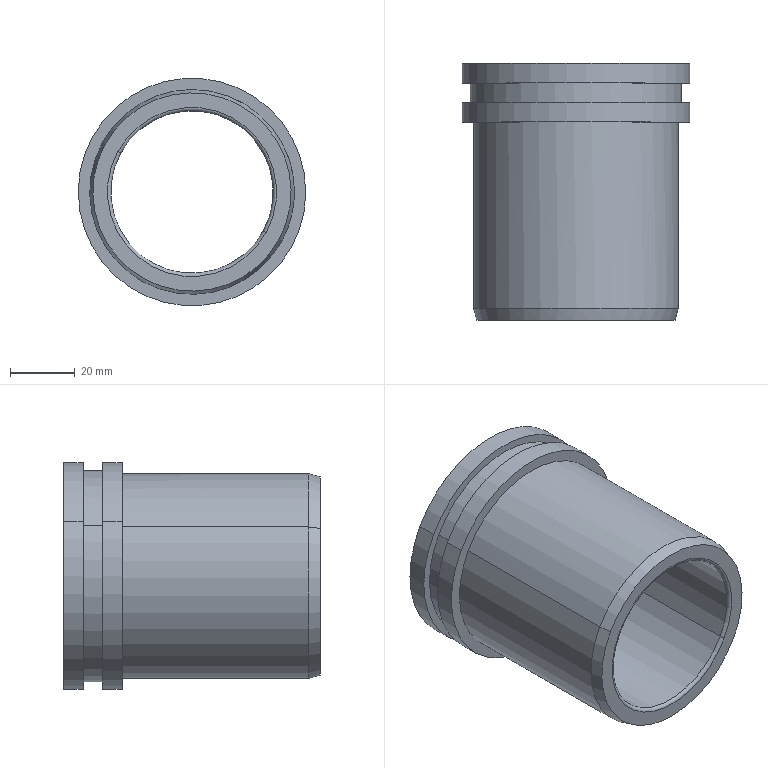Part | CATIA | 1 solid | 21 faces | box 70 x 79 x 70 mm | volume 99847 mm3 | cylinder 10 | plane 5 | torus 4 | cone 2 | commonest cylinder face diameters 70 x4 50 x2 63 x2 65 x2
STEP:
#1=CARTESIAN_POINT('',(-30.715,0.,16.78));
#2=VERTEX_POINT('',#1);
#3=CARTESIAN_POINT('',(-30.715,6.,16.78));
#4=VERTEX_POINT('',#3);
#5=CARTESIAN_POINT('',(-30.715,-21.5,16.78));
#6=DIRECTION('',(0.,1.,0.));
#7=VECTOR('',#6,1.);
#8=LINE('',#5,#7);
#9=EDGE_CURVE('',#2,#4,#8,.T.);
#10=ORIENTED_EDGE('',*,*,#9,.T.);
#11=CARTESIAN_POINT('',(30.715,6.,-16.78));
#12=VERTEX_POINT('',#11);
#13=CARTESIAN_POINT('',(0.,6.,0.));
#14=DIRECTION('',(0.,1.,0.));
#15=AXIS2_PLACEMENT_3D('',#13,#14,$);
#16=CIRCLE('',#15,35.);
#17=EDGE_CURVE('',#12,#4,#16,.T.);
#18=ORIENTED_EDGE('',*,*,#17,.F.);
#19=CARTESIAN_POINT('',(30.715,0.,-16.78));
#20=VERTEX_POINT('',#19);
#21=CARTESIAN_POINT('',(30.715,-21.5,-16.78));
#22=DIRECTION('',(0.,1.,0.));
#23=VECTOR('',#22,1.);
#24=LINE('',#21,#23);
#25=EDGE_CURVE('',#20,#12,#24,.T.);
#26=ORIENTED_EDGE('',*,*,#25,.F.);
#27=CARTESIAN_POINT('',(0.,0.,0.));
#28=DIRECTION('',(0.,1.,0.));
#29=AXIS2_PLACEMENT_3D('',#27,#28,$);
#30=CIRCLE('',#29,35.);
#31=EDGE_CURVE('',#20,#2,#30,.T.);
#32=ORIENTED_EDGE('',*,*,#31,.T.);
#33=EDGE_LOOP('',(#10,#18,#26,#32));
#34=FACE_OUTER_BOUND('',#33,.T.);
#35=CARTESIAN_POINT('',(0.,-21.5,0.));
#36=DIRECTION('',(0.,1.,0.));
#37=DIRECTION('',(0.8776,0.,-0.4794));
#38=AXIS2_PLACEMENT_3D('',#35,#36,#37);
#39=CYLINDRICAL_SURFACE('',#38,35.);
#40=ADVANCED_FACE('',(#34),#39,.T.);
#41=ORIENTED_EDGE('',*,*,#25,.T.);
#42=CARTESIAN_POINT('',(0.,6.,0.));
#43=DIRECTION('',(0.,1.,0.));
#44=AXIS2_PLACEMENT_3D('',#42,#43,$);
#45=CIRCLE('',#44,35.);
#46=EDGE_CURVE('',#4,#12,#45,.T.);
#47=ORIENTED_EDGE('',*,*,#46,.F.);
#48=ORIENTED_EDGE('',*,*,#9,.F.);
#49=CARTESIAN_POINT('',(0.,0.,0.));
#50=DIRECTION('',(0.,1.,0.));
#51=AXIS2_PLACEMENT_3D('',#49,#50,$);
#52=CIRCLE('',#51,35.);
#53=EDGE_CURVE('',#2,#20,#52,.T.);
#54=ORIENTED_EDGE('',*,*,#53,.T.);
#55=EDGE_LOOP('',(#41,#47,#48,#54));
#56=FACE_OUTER_BOUND('',#55,.T.);
#57=CARTESIAN_POINT('',(0.,-21.5,0.));
#58=DIRECTION('',(0.,1.,0.));
#59=DIRECTION('',(-0.8776,0.,0.4794));
#60=AXIS2_PLACEMENT_3D('',#57,#58,#59);
#61=CYLINDRICAL_SURFACE('',#60,35.);
#62=ADVANCED_FACE('',(#56),#61,.T.);
#63=ORIENTED_EDGE('',*,*,#46,.T.);
#64=ORIENTED_EDGE('',*,*,#17,.T.);
#65=EDGE_LOOP('',(#63,#64));
#66=FACE_OUTER_BOUND('',#65,.T.);
#67=CARTESIAN_POINT('',(28.521,6.,-15.581));
#68=VERTEX_POINT('',#67);
#69=CARTESIAN_POINT('',(-28.521,6.,15.581));
#70=VERTEX_POINT('',#69);
#71=CARTESIAN_POINT('',(0.,6.,0.));
#72=DIRECTION('',(0.,1.,0.));
#73=AXIS2_PLACEMENT_3D('',#71,#72,$);
#74=CIRCLE('',#73,32.5);
#75=EDGE_CURVE('',#68,#70,#74,.T.);
#76=ORIENTED_EDGE('',*,*,#75,.F.);
#77=CARTESIAN_POINT('',(0.,6.,0.));
#78=DIRECTION('',(0.,1.,0.));
#79=AXIS2_PLACEMENT_3D('',#77,#78,$);
#80=CIRCLE('',#79,32.5);
#81=EDGE_CURVE('',#70,#68,#80,.T.);
#82=ORIENTED_EDGE('',*,*,#81,.F.);
#83=EDGE_LOOP('',(#76,#82));
#84=FACE_BOUND('',#83,.T.);
#85=CARTESIAN_POINT('',(35.,6.,0.));
#86=DIRECTION('',(0.,1.,0.));
#87=DIRECTION('',(1.,0.,0.));
#88=AXIS2_PLACEMENT_3D('',#85,#86,#87);
#89=PLANE('',#88);
#90=ADVANCED_FACE('',(#66,#84),#89,.T.);
#91=ORIENTED_EDGE('',*,*,#31,.F.);
#92=ORIENTED_EDGE('',*,*,#53,.F.);
#93=EDGE_LOOP('',(#91,#92));
#94=FACE_OUTER_BOUND('',#93,.T.);
#95=CARTESIAN_POINT('',(-27.644,0.,15.102));
#96=VERTEX_POINT('',#95);
#97=CARTESIAN_POINT('',(27.644,0.,-15.102));
#98=VERTEX_POINT('',#97);
#99=CARTESIAN_POINT('',(0.,0.,0.));
#100=DIRECTION('',(0.,1.,0.));
#101=AXIS2_PLACEMENT_3D('',#99,#100,$);
#102=CIRCLE('',#101,31.5);
#103=EDGE_CURVE('',#96,#98,#102,.T.);
#104=ORIENTED_EDGE('',*,*,#103,.T.);
#105=CARTESIAN_POINT('',(0.,0.,0.));
#106=DIRECTION('',(0.,1.,0.));
#107=AXIS2_PLACEMENT_3D('',#105,#106,$);
#108=CIRCLE('',#107,31.5);
#109=EDGE_CURVE('',#98,#96,#108,.T.);
#110=ORIENTED_EDGE('',*,*,#109,.T.);
#111=EDGE_LOOP('',(#104,#110));
#112=FACE_BOUND('',#111,.T.);
#113=CARTESIAN_POINT('',(35.,0.,0.));
#114=DIRECTION('',(0.,1.,0.));
#115=DIRECTION('',(1.,0.,0.));
#116=AXIS2_PLACEMENT_3D('',#113,#114,#115);
#117=PLANE('',#116);
#118=ADVANCED_FACE('',(#94,#112),#117,.F.);
#119=CARTESIAN_POINT('',(-28.521,12.,15.581));
#120=VERTEX_POINT('',#119);
#121=CARTESIAN_POINT('',(-28.521,-21.5,15.581));
#122=DIRECTION('',(0.,1.,0.));
#123=VECTOR('',#122,1.);
#124=LINE('',#121,#123);
#125=EDGE_CURVE('',#70,#120,#124,.T.);
#126=ORIENTED_EDGE('',*,*,#125,.T.);
#127=CARTESIAN_POINT('',(28.521,12.,-15.581));
#128=VERTEX_POINT('',#127);
#129=CARTESIAN_POINT('',(0.,12.,0.));
#130=DIRECTION('',(0.,1.,0.));
#131=AXIS2_PLACEMENT_3D('',#129,#130,$);
#132=CIRCLE('',#131,32.5);
#133=EDGE_CURVE('',#128,#120,#132,.T.);
#134=ORIENTED_EDGE('',*,*,#133,.F.);
#135=CARTESIAN_POINT('',(28.521,-21.5,-15.581));
#136=DIRECTION('',(0.,1.,0.));
#137=VECTOR('',#136,1.);
#138=LINE('',#135,#137);
#139=EDGE_CURVE('',#68,#128,#138,.T.);
#140=ORIENTED_EDGE('',*,*,#139,.F.);
#141=ORIENTED_EDGE('',*,*,#75,.T.);
#142=EDGE_LOOP('',(#126,#134,#140,#141));
#143=FACE_OUTER_BOUND('',#142,.T.);
#144=CARTESIAN_POINT('',(0.,-21.5,0.));
#145=DIRECTION('',(0.,1.,0.));
#146=DIRECTION('',(0.8776,0.,-0.4794));
#147=AXIS2_PLACEMENT_3D('',#144,#145,#146);
#148=CYLINDRICAL_SURFACE('',#147,32.5);
#149=ADVANCED_FACE('',(#143),#148,.T.);
#150=ORIENTED_EDGE('',*,*,#139,.T.);
#151=CARTESIAN_POINT('',(0.,12.,0.));
#152=DIRECTION('',(0.,1.,0.));
#153=AXIS2_PLACEMENT_3D('',#151,#152,$);
#154=CIRCLE('',#153,32.5);
#155=EDGE_CURVE('',#120,#128,#154,.T.);
#156=ORIENTED_EDGE('',*,*,#155,.F.);
#157=ORIENTED_EDGE('',*,*,#125,.F.);
#158=ORIENTED_EDGE('',*,*,#81,.T.);
#159=EDGE_LOOP('',(#150,#156,#157,#158));
#160=FACE_OUTER_BOUND('',#159,.T.);
#161=CARTESIAN_POINT('',(0.,-21.5,0.));
#162=DIRECTION('',(0.,1.,0.));
#163=DIRECTION('',(-0.8776,0.,0.4794));
#164=AXIS2_PLACEMENT_3D('',#161,#162,#163);
#165=CYLINDRICAL_SURFACE('',#164,32.5);
#166=ADVANCED_FACE('',(#160),#165,.T.);
#167=CARTESIAN_POINT('',(27.644,-57.268,-15.102));
#168=VERTEX_POINT('',#167);
#169=CARTESIAN_POINT('',(27.644,-21.5,-15.102));
#170=DIRECTION('',(0.,1.,0.));
#171=VECTOR('',#170,1.);
#172=LINE('',#169,#171);
#173=EDGE_CURVE('',#168,#98,#172,.T.);
#174=ORIENTED_EDGE('',*,*,#173,.T.);
#175=ORIENTED_EDGE('',*,*,#103,.F.);
#176=CARTESIAN_POINT('',(-27.644,-57.268,15.102));
#177=VERTEX_POINT('',#176);
#178=CARTESIAN_POINT('',(-27.644,-21.5,15.102));
#179=DIRECTION('',(0.,1.,0.));
#180=VECTOR('',#179,1.);
#181=LINE('',#178,#180);
#182=EDGE_CURVE('',#177,#96,#181,.T.);
#183=ORIENTED_EDGE('',*,*,#182,.F.);
#184=CARTESIAN_POINT('',(-27.644,-57.268,15.102));
#185=CARTESIAN_POINT('',(-25.272,-57.268,19.444));
#186=CARTESIAN_POINT('',(-22.047,-57.268,23.321));
#187=CARTESIAN_POINT('',(-18.091,-57.268,26.507));
#188=CARTESIAN_POINT('',(-9.142,-57.268,31.158));
#189=CARTESIAN_POINT('',(0.9008,-57.268,32.08));
#190=CARTESIAN_POINT('',(5.952,-57.268,31.536));
#191=CARTESIAN_POINT('',(15.568,-57.268,28.496));
#192=CARTESIAN_POINT('',(23.321,-57.268,22.047));
#193=CARTESIAN_POINT('',(26.507,-57.268,18.091));
#194=CARTESIAN_POINT('',(31.158,-57.268,9.142));
#195=CARTESIAN_POINT('',(32.08,-57.268,-0.9008));
#196=CARTESIAN_POINT('',(31.536,-57.268,-5.952));
#197=CARTESIAN_POINT('',(30.016,-57.268,-10.76));
#198=CARTESIAN_POINT('',(27.644,-57.268,-15.102));
#199=B_SPLINE_CURVE_WITH_KNOTS('',5,(#184,#185,#186,#187,#188,#189,#190,#191,#192,#193,#194,#195,#196,#197,#198),.UNSPECIFIED.,.F.,.U.,(6,3,3,3,6),(-49.48,-24.74,0.,24.74,49.48),.UNSPECIFIED.);
#200=EDGE_CURVE('',#177,#168,#199,.T.);
#201=ORIENTED_EDGE('',*,*,#200,.T.);
#202=EDGE_LOOP('',(#174,#175,#183,#201));
#203=FACE_OUTER_BOUND('',#202,.T.);
#204=CARTESIAN_POINT('',(0.,-21.5,0.));
#205=DIRECTION('',(0.,1.,0.));
#206=DIRECTION('',(-0.8776,0.,0.4794));
#207=AXIS2_PLACEMENT_3D('',#204,#205,#206);
#208=CYLINDRICAL_SURFACE('',#207,31.5);
#209=ADVANCED_FACE('',(#203),#208,.T.);
#210=ORIENTED_EDGE('',*,*,#182,.T.);
#211=ORIENTED_EDGE('',*,*,#109,.F.);
#212=ORIENTED_EDGE('',*,*,#173,.F.);
#213=CARTESIAN_POINT('',(0.,-57.268,0.));
#214=DIRECTION('',(0.,1.,0.));
#215=AXIS2_PLACEMENT_3D('',#213,#214,$);
#216=CIRCLE('',#215,31.5);
#217=EDGE_CURVE('',#168,#177,#216,.T.);
#218=ORIENTED_EDGE('',*,*,#217,.T.);
#219=EDGE_LOOP('',(#210,#211,#212,#218));
#220=FACE_OUTER_BOUND('',#219,.T.);
#221=CARTESIAN_POINT('',(0.,-21.5,0.));
#222=DIRECTION('',(0.,1.,0.));
#223=DIRECTION('',(0.8776,0.,-0.4794));
#224=AXIS2_PLACEMENT_3D('',#221,#222,#223);
#225=CYLINDRICAL_SURFACE('',#224,31.5);
#226=ADVANCED_FACE('',(#220),#225,.T.);
#227=CARTESIAN_POINT('',(30.715,12.,-16.78));
#228=VERTEX_POINT('',#227);
#229=CARTESIAN_POINT('',(-30.715,12.,16.78));
#230=VERTEX_POINT('',#229);
#231=CARTESIAN_POINT('',(0.,12.,0.));
#232=DIRECTION('',(0.,1.,0.));
#233=AXIS2_PLACEMENT_3D('',#231,#232,$);
#234=CIRCLE('',#233,35.);
#235=EDGE_CURVE('',#228,#230,#234,.T.);
#236=ORIENTED_EDGE('',*,*,#235,.F.);
#237=CARTESIAN_POINT('',(0.,12.,0.));
#238=DIRECTION('',(0.,1.,0.));
#239=AXIS2_PLACEMENT_3D('',#237,#238,$);
#240=CIRCLE('',#239,35.);
#241=EDGE_CURVE('',#230,#228,#240,.T.);
#242=ORIENTED_EDGE('',*,*,#241,.F.);
#243=EDGE_LOOP('',(#236,#242));
#244=FACE_OUTER_BOUND('',#243,.T.);
#245=ORIENTED_EDGE('',*,*,#155,.T.);
#246=ORIENTED_EDGE('',*,*,#133,.T.);
#247=EDGE_LOOP('',(#245,#246));
#248=FACE_BOUND('',#247,.T.);
#249=CARTESIAN_POINT('',(35.,12.,0.));
#250=DIRECTION('',(0.,1.,0.));
#251=DIRECTION('',(1.,0.,0.));
#252=AXIS2_PLACEMENT_3D('',#249,#250,#251);
#253=PLANE('',#252);
#254=ADVANCED_FACE('',(#244,#248),#253,.F.);
#255=CARTESIAN_POINT('',(26.766,-61.,-14.622));
#256=VERTEX_POINT('',#255);
#257=CARTESIAN_POINT('',(113580.923,482844.999,-62049.541));
#258=DIRECTION('',(0.2271,0.9659,-0.1241));
#259=VECTOR('',#258,1.);
#260=LINE('',#257,#259);
#261=EDGE_CURVE('',#256,#168,#260,.T.);
#262=ORIENTED_EDGE('',*,*,#261,.T.);
#263=ORIENTED_EDGE('',*,*,#200,.F.);
#264=CARTESIAN_POINT('',(-26.766,-61.,14.622));
#265=VERTEX_POINT('',#264);
#266=CARTESIAN_POINT('',(-113580.923,482844.999,62049.541));
#267=DIRECTION('',(-0.2271,0.9659,0.1241));
#268=VECTOR('',#267,1.);
#269=LINE('',#266,#268);
#270=EDGE_CURVE('',#265,#177,#269,.T.);
#271=ORIENTED_EDGE('',*,*,#270,.F.);
#272=CARTESIAN_POINT('',(0.,-61.,0.));
#273=DIRECTION('',(0.,1.,0.));
#274=AXIS2_PLACEMENT_3D('',#272,#273,$);
#275=CIRCLE('',#274,30.5);
#276=EDGE_CURVE('',#265,#256,#275,.T.);
#277=ORIENTED_EDGE('',*,*,#276,.T.);
#278=EDGE_LOOP('',(#262,#263,#271,#277));
#279=FACE_OUTER_BOUND('',#278,.T.);
#280=CARTESIAN_POINT('',(0.,-61.,0.));
#281=DIRECTION('',(0.,1.,0.));
#282=DIRECTION('',(-0.8776,0.,0.4794));
#283=AXIS2_PLACEMENT_3D('',#280,#281,#282);
#284=CONICAL_SURFACE('',#283,30.5,0.2618);
#285=ADVANCED_FACE('',(#279),#284,.T.);
#286=ORIENTED_EDGE('',*,*,#270,.T.);
#287=ORIENTED_EDGE('',*,*,#217,.F.);
#288=ORIENTED_EDGE('',*,*,#261,.F.);
#289=CARTESIAN_POINT('',(0.,-61.,0.));
#290=DIRECTION('',(0.,1.,0.));
#291=AXIS2_PLACEMENT_3D('',#289,#290,$);
#292=CIRCLE('',#291,30.5);
#293=EDGE_CURVE('',#256,#265,#292,.T.);
#294=ORIENTED_EDGE('',*,*,#293,.T.);
#295=EDGE_LOOP('',(#286,#287,#288,#294));
#296=FACE_OUTER_BOUND('',#295,.T.);
#297=CARTESIAN_POINT('',(0.,-61.,0.));
#298=DIRECTION('',(0.,1.,0.));
#299=DIRECTION('',(0.8776,0.,-0.4794));
#300=AXIS2_PLACEMENT_3D('',#297,#298,#299);
#301=CONICAL_SURFACE('',#300,30.5,0.2618);
#302=ADVANCED_FACE('',(#296),#301,.T.);
#303=CARTESIAN_POINT('',(-30.715,18.,16.78));
#304=VERTEX_POINT('',#303);
#305=CARTESIAN_POINT('',(-30.715,-21.5,16.78));
#306=DIRECTION('',(0.,1.,0.));
#307=VECTOR('',#306,1.);
#308=LINE('',#305,#307);
#309=EDGE_CURVE('',#230,#304,#308,.T.);
#310=ORIENTED_EDGE('',*,*,#309,.T.);
#311=CARTESIAN_POINT('',(30.715,18.,-16.78));
#312=VERTEX_POINT('',#311);
#313=CARTESIAN_POINT('',(0.,18.,0.));
#314=DIRECTION('',(0.,1.,0.));
#315=AXIS2_PLACEMENT_3D('',#313,#314,$);
#316=CIRCLE('',#315,35.);
#317=EDGE_CURVE('',#312,#304,#316,.T.);
#318=ORIENTED_EDGE('',*,*,#317,.F.);
#319=CARTESIAN_POINT('',(30.715,-21.5,-16.78));
#320=DIRECTION('',(0.,1.,0.));
#321=VECTOR('',#320,1.);
#322=LINE('',#319,#321);
#323=EDGE_CURVE('',#228,#312,#322,.T.);
#324=ORIENTED_EDGE('',*,*,#323,.F.);
#325=ORIENTED_EDGE('',*,*,#235,.T.);
#326=EDGE_LOOP('',(#310,#318,#324,#325));
#327=FACE_OUTER_BOUND('',#326,.T.);
#328=ADVANCED_FACE('',(#327),#39,.T.);
#329=ORIENTED_EDGE('',*,*,#323,.T.);
#330=CARTESIAN_POINT('',(0.,18.,0.));
#331=DIRECTION('',(0.,1.,0.));
#332=AXIS2_PLACEMENT_3D('',#330,#331,$);
#333=CIRCLE('',#332,35.);
#334=EDGE_CURVE('',#304,#312,#333,.T.);
#335=ORIENTED_EDGE('',*,*,#334,.F.);
#336=ORIENTED_EDGE('',*,*,#309,.F.);
#337=ORIENTED_EDGE('',*,*,#241,.T.);
#338=EDGE_LOOP('',(#329,#335,#336,#337));
#339=FACE_OUTER_BOUND('',#338,.T.);
#340=ADVANCED_FACE('',(#339),#61,.T.);
#341=ORIENTED_EDGE('',*,*,#293,.F.);
#342=ORIENTED_EDGE('',*,*,#276,.F.);
#343=EDGE_LOOP('',(#341,#342));
#344=FACE_OUTER_BOUND('',#343,.T.);
#345=CARTESIAN_POINT('',(-22.817,-61.,12.465));
#346=VERTEX_POINT('',#345);
#347=CARTESIAN_POINT('',(22.817,-61.,-12.465));
#348=VERTEX_POINT('',#347);
#349=CARTESIAN_POINT('',(0.,-61.,0.));
#350=DIRECTION('',(0.,1.,0.));
#351=AXIS2_PLACEMENT_3D('',#349,#350,$);
#352=CIRCLE('',#351,26.);
#353=EDGE_CURVE('',#346,#348,#352,.T.);
#354=ORIENTED_EDGE('',*,*,#353,.T.);
#355=CARTESIAN_POINT('',(0.,-61.,0.));
#356=DIRECTION('',(0.,1.,0.));
#357=AXIS2_PLACEMENT_3D('',#355,#356,$);
#358=CIRCLE('',#357,26.);
#359=EDGE_CURVE('',#348,#346,#358,.T.);
#360=ORIENTED_EDGE('',*,*,#359,.T.);
#361=EDGE_LOOP('',(#354,#360));
#362=FACE_BOUND('',#361,.T.);
#363=CARTESIAN_POINT('',(26.,-61.,0.));
#364=DIRECTION('',(0.,1.,0.));
#365=DIRECTION('',(1.,0.,0.));
#366=AXIS2_PLACEMENT_3D('',#363,#364,#365);
#367=PLANE('',#366);
#368=ADVANCED_FACE('',(#344,#362),#367,.F.);
#369=ORIENTED_EDGE('',*,*,#334,.T.);
#370=ORIENTED_EDGE('',*,*,#317,.T.);
#371=EDGE_LOOP('',(#369,#370));
#372=FACE_OUTER_BOUND('',#371,.T.);
#373=CARTESIAN_POINT('',(26.327,18.,-14.383));
#374=VERTEX_POINT('',#373);
#375=CARTESIAN_POINT('',(-26.327,18.,14.383));
#376=VERTEX_POINT('',#375);
#377=CARTESIAN_POINT('',(0.,18.,0.));
#378=DIRECTION('',(0.,1.,0.));
#379=AXIS2_PLACEMENT_3D('',#377,#378,$);
#380=CIRCLE('',#379,30.);
#381=EDGE_CURVE('',#374,#376,#380,.T.);
#382=ORIENTED_EDGE('',*,*,#381,.F.);
#383=CARTESIAN_POINT('',(0.,18.,0.));
#384=DIRECTION('',(0.,1.,0.));
#385=AXIS2_PLACEMENT_3D('',#383,#384,$);
#386=CIRCLE('',#385,30.);
#387=EDGE_CURVE('',#376,#374,#386,.T.);
#388=ORIENTED_EDGE('',*,*,#387,.F.);
#389=EDGE_LOOP('',(#382,#388));
#390=FACE_BOUND('',#389,.T.);
#391=CARTESIAN_POINT('',(30.,18.,0.));
#392=DIRECTION('',(0.,1.,0.));
#393=DIRECTION('',(1.,0.,0.));
#394=AXIS2_PLACEMENT_3D('',#391,#392,#393);
#395=PLANE('',#394);
#396=ADVANCED_FACE('',(#372,#390),#395,.T.);
#397=CARTESIAN_POINT('',(21.94,-60.,-11.986));
#398=VERTEX_POINT('',#397);
#399=CARTESIAN_POINT('',(22.817,-60.,-12.465));
#400=DIRECTION('',(0.4794,0.,0.8776));
#401=AXIS2_PLACEMENT_3D('',#399,#400,$);
#402=CIRCLE('',#401,1.);
#403=EDGE_CURVE('',#398,#348,#402,.T.);
#404=ORIENTED_EDGE('',*,*,#403,.T.);
#405=ORIENTED_EDGE('',*,*,#353,.F.);
#406=CARTESIAN_POINT('',(-21.94,-60.,11.986));
#407=VERTEX_POINT('',#406);
#408=CARTESIAN_POINT('',(-22.817,-60.,12.465));
#409=DIRECTION('',(-0.4794,0.,-0.8776));
#410=AXIS2_PLACEMENT_3D('',#408,#409,$);
#411=CIRCLE('',#410,1.);
#412=EDGE_CURVE('',#407,#346,#411,.T.);
#413=ORIENTED_EDGE('',*,*,#412,.F.);
#414=CARTESIAN_POINT('',(0.,-60.,0.));
#415=DIRECTION('',(0.,1.,0.));
#416=AXIS2_PLACEMENT_3D('',#414,#415,$);
#417=CIRCLE('',#416,25.);
#418=EDGE_CURVE('',#407,#398,#417,.T.);
#419=ORIENTED_EDGE('',*,*,#418,.T.);
#420=EDGE_LOOP('',(#404,#405,#413,#419));
#421=FACE_OUTER_BOUND('',#420,.T.);
#422=CARTESIAN_POINT('',(0.,-60.,0.));
#423=DIRECTION('',(0.,1.,0.));
#424=DIRECTION('',(-0.8776,0.,0.4794));
#425=AXIS2_PLACEMENT_3D('',#422,#423,#424);
#426=TOROIDAL_SURFACE('',#425,26.,1.);
#427=ADVANCED_FACE('',(#421),#426,.T.);
#428=ORIENTED_EDGE('',*,*,#412,.T.);
#429=ORIENTED_EDGE('',*,*,#359,.F.);
#430=ORIENTED_EDGE('',*,*,#403,.F.);
#431=CARTESIAN_POINT('',(0.,-60.,0.));
#432=DIRECTION('',(0.,1.,0.));
#433=AXIS2_PLACEMENT_3D('',#431,#432,$);
#434=CIRCLE('',#433,25.);
#435=EDGE_CURVE('',#398,#407,#434,.T.);
#436=ORIENTED_EDGE('',*,*,#435,.T.);
#437=EDGE_LOOP('',(#428,#429,#430,#436));
#438=FACE_OUTER_BOUND('',#437,.T.);
#439=CARTESIAN_POINT('',(0.,-60.,0.));
#440=DIRECTION('',(0.,1.,0.));
#441=DIRECTION('',(0.8776,0.,-0.4794));
#442=AXIS2_PLACEMENT_3D('',#439,#440,#441);
#443=TOROIDAL_SURFACE('',#442,26.,1.);
#444=ADVANCED_FACE('',(#438),#443,.T.);
#445=CARTESIAN_POINT('',(-21.94,13.,11.986));
#446=VERTEX_POINT('',#445);
#447=CARTESIAN_POINT('',(-26.327,13.,14.383));
#448=DIRECTION('',(-0.4794,0.,-0.8776));
#449=AXIS2_PLACEMENT_3D('',#447,#448,$);
#450=CIRCLE('',#449,5.);
#451=EDGE_CURVE('',#376,#446,#450,.T.);
#452=ORIENTED_EDGE('',*,*,#451,.T.);
#453=CARTESIAN_POINT('',(21.94,13.,-11.986));
#454=VERTEX_POINT('',#453);
#455=CARTESIAN_POINT('',(0.,13.,0.));
#456=DIRECTION('',(0.,1.,0.));
#457=AXIS2_PLACEMENT_3D('',#455,#456,$);
#458=CIRCLE('',#457,25.);
#459=EDGE_CURVE('',#454,#446,#458,.T.);
#460=ORIENTED_EDGE('',*,*,#459,.F.);
#461=CARTESIAN_POINT('',(26.327,13.,-14.383));
#462=DIRECTION('',(0.4794,0.,0.8776));
#463=AXIS2_PLACEMENT_3D('',#461,#462,$);
#464=CIRCLE('',#463,5.);
#465=EDGE_CURVE('',#374,#454,#464,.T.);
#466=ORIENTED_EDGE('',*,*,#465,.F.);
#467=ORIENTED_EDGE('',*,*,#381,.T.);
#468=EDGE_LOOP('',(#452,#460,#466,#467));
#469=FACE_OUTER_BOUND('',#468,.T.);
#470=CARTESIAN_POINT('',(0.,13.,0.));
#471=DIRECTION('',(0.,1.,0.));
#472=DIRECTION('',(0.8776,0.,-0.4794));
#473=AXIS2_PLACEMENT_3D('',#470,#471,#472);
#474=TOROIDAL_SURFACE('',#473,30.,5.);
#475=ADVANCED_FACE('',(#469),#474,.T.);
#476=ORIENTED_EDGE('',*,*,#465,.T.);
#477=CARTESIAN_POINT('',(0.,13.,0.));
#478=DIRECTION('',(0.,1.,0.));
#479=AXIS2_PLACEMENT_3D('',#477,#478,$);
#480=CIRCLE('',#479,25.);
#481=EDGE_CURVE('',#446,#454,#480,.T.);
#482=ORIENTED_EDGE('',*,*,#481,.F.);
#483=ORIENTED_EDGE('',*,*,#451,.F.);
#484=ORIENTED_EDGE('',*,*,#387,.T.);
#485=EDGE_LOOP('',(#476,#482,#483,#484));
#486=FACE_OUTER_BOUND('',#485,.T.);
#487=CARTESIAN_POINT('',(0.,13.,0.));
#488=DIRECTION('',(0.,1.,0.));
#489=DIRECTION('',(-0.8776,0.,0.4794));
#490=AXIS2_PLACEMENT_3D('',#487,#488,#489);
#491=TOROIDAL_SURFACE('',#490,30.,5.);
#492=ADVANCED_FACE('',(#486),#491,.T.);
#493=CARTESIAN_POINT('',(21.94,-21.5,-11.986));
#494=DIRECTION('',(0.,1.,0.));
#495=VECTOR('',#494,1.);
#496=LINE('',#493,#495);
#497=EDGE_CURVE('',#454,#398,#496,.F.);
#498=ORIENTED_EDGE('',*,*,#497,.T.);
#499=ORIENTED_EDGE('',*,*,#418,.F.);
#500=CARTESIAN_POINT('',(-21.94,-21.5,11.986));
#501=DIRECTION('',(0.,1.,0.));
#502=VECTOR('',#501,1.);
#503=LINE('',#500,#502);
#504=EDGE_CURVE('',#446,#407,#503,.F.);
#505=ORIENTED_EDGE('',*,*,#504,.F.);
#506=ORIENTED_EDGE('',*,*,#481,.T.);
#507=EDGE_LOOP('',(#498,#499,#505,#506));
#508=FACE_OUTER_BOUND('',#507,.T.);
#509=CARTESIAN_POINT('',(0.,-21.5,0.));
#510=DIRECTION('',(0.,1.,0.));
#511=DIRECTION('',(-0.8776,0.,0.4794));
#512=AXIS2_PLACEMENT_3D('',#509,#510,#511);
#513=CYLINDRICAL_SURFACE('',#512,25.);
#514=ADVANCED_FACE('',(#508),#513,.F.);
#515=ORIENTED_EDGE('',*,*,#504,.T.);
#516=ORIENTED_EDGE('',*,*,#435,.F.);
#517=ORIENTED_EDGE('',*,*,#497,.F.);
#518=ORIENTED_EDGE('',*,*,#459,.T.);
#519=EDGE_LOOP('',(#515,#516,#517,#518));
#520=FACE_OUTER_BOUND('',#519,.T.);
#521=CARTESIAN_POINT('',(0.,-21.5,0.));
#522=DIRECTION('',(0.,1.,0.));
#523=DIRECTION('',(0.8776,0.,-0.4794));
#524=AXIS2_PLACEMENT_3D('',#521,#522,#523);
#525=CYLINDRICAL_SURFACE('',#524,25.);
#526=ADVANCED_FACE('',(#520),#525,.F.);
#527=CLOSED_SHELL('',(#40,#62,#90,#118,#149,#166,#209,#226,#254,#285,#302,#328,#340,#368,#396,#427,#444,#475,#492,#514,#526));
#528=MANIFOLD_SOLID_BREP('',#527);
#529=(LENGTH_UNIT()NAMED_UNIT(*)SI_UNIT(.MILLI.,.METRE.));
#530=UNCERTAINTY_MEASURE_WITH_UNIT(LENGTH_MEASURE(0.005),#529,'','');
#531=(NAMED_UNIT(*)PLANE_ANGLE_UNIT()SI_UNIT($,.RADIAN.));
#532=(NAMED_UNIT(*)SI_UNIT($,.STERADIAN.)SOLID_ANGLE_UNIT());
#533=(GEOMETRIC_REPRESENTATION_CONTEXT(3)GLOBAL_UNCERTAINTY_ASSIGNED_CONTEXT((#530))GLOBAL_UNIT_ASSIGNED_CONTEXT((#529,#531,#532))REPRESENTATION_CONTEXT('',''));
#534=ADVANCED_BREP_SHAPE_REPRESENTATION('',(#528),#533);